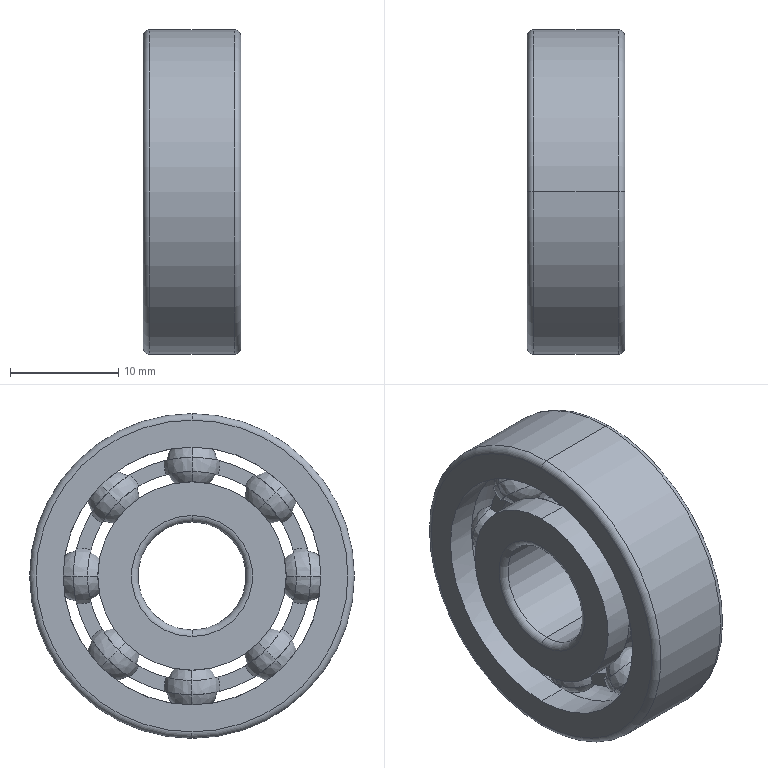Part | SolidWorks | features Revolution 5, CirPattern 2, RevCut 2 | 1 solid | 132 faces | box 9 x 30 x 30 mm | volume 4054 mm3 | sphere 64 | torus 32 | plane 20 | cylinder 16 | commonest cylinder face diameters 17.4 x4 23.8 x4 10 x2 19.29 x2 21.91 x2 30 x2